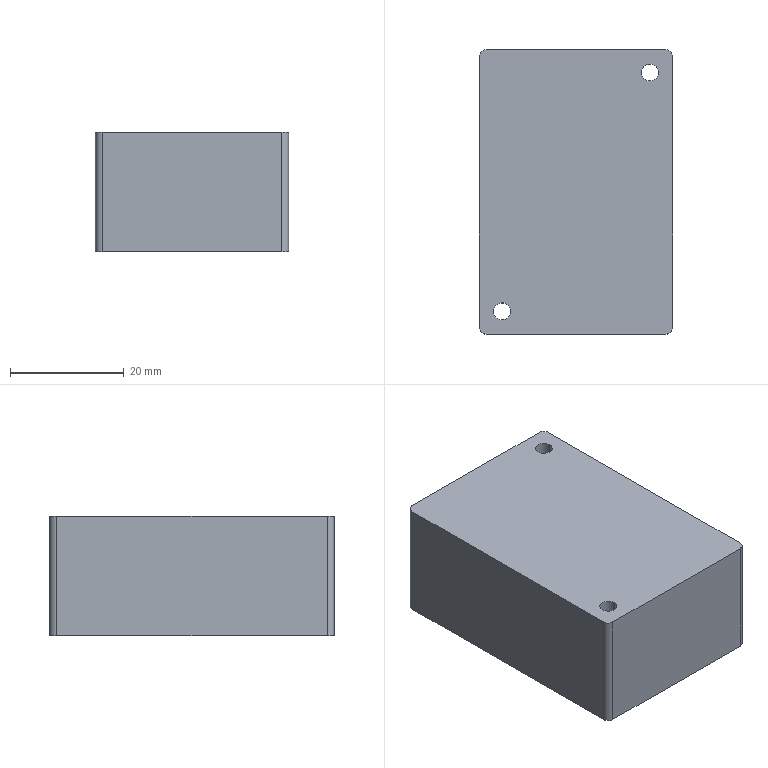Part | STEP file | 4V430C_15_Valve_Cover | 1 solid | 14 faces | box 34 x 50 x 21 mm | volume 35377 mm3 | cylinder 8 | plane 6 | commonest cylinder face diameters 2.4 x4 3 x4
STEP:
#1=CARTESIAN_POINT('',(0.,0.,0.));
#2=DIRECTION('',(0.,0.,1.));
#3=DIRECTION('',(1.,0.,0.));
#4=AXIS2_PLACEMENT_3D('',#1,#2,#3);
#5=CARTESIAN_POINT('',(-11.5,-21.,-21.));
#6=VERTEX_POINT('',#5);
#7=CARTESIAN_POINT('',(-11.5,-21.,0.));
#8=VERTEX_POINT('',#7);
#9=CARTESIAN_POINT('',(-11.5,-21.,-21.));
#10=DIRECTION('',(0.,0.,1.));
#11=VECTOR('',#10,1.);
#12=LINE('',#9,#11);
#13=CARTESIAN_POINT('',(-13.,-21.,-21.));
#14=DIRECTION('',(0.,0.,1.));
#15=DIRECTION('',(1.,0.,0.));
#16=AXIS2_PLACEMENT_3D('',#13,#14,#15);
#17=CYLINDRICAL_SURFACE('',#16,1.5);
#18=CARTESIAN_POINT('',(6.283,0.));
#19=DIRECTION('',(0.,1.));
#20=VECTOR('',#19,1.);
#21=LINE('',#18,#20);
#22=(GEOMETRIC_REPRESENTATION_CONTEXT(2)PARAMETRIC_REPRESENTATION_CONTEXT()REPRESENTATION_CONTEXT('',''));
#23=DEFINITIONAL_REPRESENTATION('',(#21),#22);
#24=PCURVE('',#17,#23);
#25=CARTESIAN_POINT('',(-13.,-21.,-21.));
#26=DIRECTION('',(0.,0.,1.));
#27=DIRECTION('',(1.,0.,0.));
#28=AXIS2_PLACEMENT_3D('',#25,#26,#27);
#29=CYLINDRICAL_SURFACE('',#28,1.5);
#30=CARTESIAN_POINT('',(0.,0.));
#31=DIRECTION('',(0.,1.));
#32=VECTOR('',#31,1.);
#33=LINE('',#30,#32);
#34=(GEOMETRIC_REPRESENTATION_CONTEXT(2)PARAMETRIC_REPRESENTATION_CONTEXT()REPRESENTATION_CONTEXT('',''));
#35=DEFINITIONAL_REPRESENTATION('',(#33),#34);
#36=PCURVE('',#29,#35);
#37=SURFACE_CURVE('',#12,(#24,#36),.PCURVE_S1.);
#38=EDGE_CURVE('',#6,#8,#37,.T.);
#39=ORIENTED_EDGE('',*,*,#38,.T.);
#40=CARTESIAN_POINT('',(-14.5,-21.,0.));
#41=VERTEX_POINT('',#40);
#42=CARTESIAN_POINT('',(-13.,-21.,0.));
#43=DIRECTION('',(0.,0.,1.));
#44=DIRECTION('',(1.,0.,0.));
#45=AXIS2_PLACEMENT_3D('',#42,#43,#44);
#46=CIRCLE('',#45,1.5);
#47=CARTESIAN_POINT('',(0.,21.));
#48=DIRECTION('',(1.,0.));
#49=VECTOR('',#48,1.);
#50=LINE('',#47,#49);
#51=(GEOMETRIC_REPRESENTATION_CONTEXT(2)PARAMETRIC_REPRESENTATION_CONTEXT()REPRESENTATION_CONTEXT('',''));
#52=DEFINITIONAL_REPRESENTATION('',(#50),#51);
#53=PCURVE('',#17,#52);
#54=CARTESIAN_POINT('',(-15.8,-23.8,0.));
#55=DIRECTION('',(0.,0.,1.));
#56=DIRECTION('',(1.,0.,0.));
#57=AXIS2_PLACEMENT_3D('',#54,#55,#56);
#58=PLANE('',#57);
#59=CARTESIAN_POINT('',(2.8,2.8));
#60=DIRECTION('',(1.,0.));
#61=AXIS2_PLACEMENT_2D('',#59,#60);
#62=CIRCLE('',#61,1.5);
#63=(GEOMETRIC_REPRESENTATION_CONTEXT(2)PARAMETRIC_REPRESENTATION_CONTEXT()REPRESENTATION_CONTEXT('',''));
#64=DEFINITIONAL_REPRESENTATION('',(#62),#63);
#65=PCURVE('',#58,#64);
#66=SURFACE_CURVE('',#46,(#53,#65),.PCURVE_S1.);
#67=EDGE_CURVE('',#41,#8,#66,.T.);
#68=ORIENTED_EDGE('',*,*,#67,.F.);
#69=CARTESIAN_POINT('',(-14.5,-21.,-21.));
#70=VERTEX_POINT('',#69);
#71=CARTESIAN_POINT('',(-14.5,-21.,-21.));
#72=DIRECTION('',(0.,0.,1.));
#73=VECTOR('',#72,1.);
#74=LINE('',#71,#73);
#75=CARTESIAN_POINT('',(3.142,0.));
#76=DIRECTION('',(0.,1.));
#77=VECTOR('',#76,1.);
#78=LINE('',#75,#77);
#79=(GEOMETRIC_REPRESENTATION_CONTEXT(2)PARAMETRIC_REPRESENTATION_CONTEXT()REPRESENTATION_CONTEXT('',''));
#80=DEFINITIONAL_REPRESENTATION('',(#78),#79);
#81=PCURVE('',#17,#80);
#82=CARTESIAN_POINT('',(3.142,0.));
#83=DIRECTION('',(0.,1.));
#84=VECTOR('',#83,1.);
#85=LINE('',#82,#84);
#86=(GEOMETRIC_REPRESENTATION_CONTEXT(2)PARAMETRIC_REPRESENTATION_CONTEXT()REPRESENTATION_CONTEXT('',''));
#87=DEFINITIONAL_REPRESENTATION('',(#85),#86);
#88=PCURVE('',#29,#87);
#89=SURFACE_CURVE('',#74,(#81,#88),.PCURVE_S1.);
#90=EDGE_CURVE('',#70,#41,#89,.T.);
#91=ORIENTED_EDGE('',*,*,#90,.F.);
#92=CARTESIAN_POINT('',(-13.,-21.,-21.));
#93=DIRECTION('',(0.,0.,1.));
#94=DIRECTION('',(1.,0.,0.));
#95=AXIS2_PLACEMENT_3D('',#92,#93,#94);
#96=CIRCLE('',#95,1.5);
#97=CARTESIAN_POINT('',(0.,0.));
#98=DIRECTION('',(1.,0.));
#99=VECTOR('',#98,1.);
#100=LINE('',#97,#99);
#101=(GEOMETRIC_REPRESENTATION_CONTEXT(2)PARAMETRIC_REPRESENTATION_CONTEXT()REPRESENTATION_CONTEXT('',''));
#102=DEFINITIONAL_REPRESENTATION('',(#100),#101);
#103=PCURVE('',#17,#102);
#104=CARTESIAN_POINT('',(-15.8,-23.8,-21.));
#105=DIRECTION('',(0.,0.,1.));
#106=DIRECTION('',(1.,0.,0.));
#107=AXIS2_PLACEMENT_3D('',#104,#105,#106);
#108=PLANE('',#107);
#109=CARTESIAN_POINT('',(2.8,2.8));
#110=DIRECTION('',(1.,0.));
#111=AXIS2_PLACEMENT_2D('',#109,#110);
#112=CIRCLE('',#111,1.5);
#113=(GEOMETRIC_REPRESENTATION_CONTEXT(2)PARAMETRIC_REPRESENTATION_CONTEXT()REPRESENTATION_CONTEXT('',''));
#114=DEFINITIONAL_REPRESENTATION('',(#112),#113);
#115=PCURVE('',#108,#114);
#116=SURFACE_CURVE('',#96,(#103,#115),.PCURVE_S1.);
#117=EDGE_CURVE('',#70,#6,#116,.T.);
#118=ORIENTED_EDGE('',*,*,#117,.T.);
#119=EDGE_LOOP('',(#39,#68,#91,#118));
#120=FACE_BOUND('',#119,.F.);
#121=ADVANCED_FACE('',(#120),#17,.F.);
#122=CARTESIAN_POINT('',(14.5,21.,-21.));
#123=VERTEX_POINT('',#122);
#124=CARTESIAN_POINT('',(14.5,21.,0.));
#125=VERTEX_POINT('',#124);
#126=CARTESIAN_POINT('',(14.5,21.,-21.));
#127=DIRECTION('',(0.,0.,1.));
#128=VECTOR('',#127,1.);
#129=LINE('',#126,#128);
#130=CARTESIAN_POINT('',(13.,21.,-21.));
#131=DIRECTION('',(0.,0.,1.));
#132=DIRECTION('',(1.,0.,0.));
#133=AXIS2_PLACEMENT_3D('',#130,#131,#132);
#134=CYLINDRICAL_SURFACE('',#133,1.5);
#135=CARTESIAN_POINT('',(6.283,0.));
#136=DIRECTION('',(0.,1.));
#137=VECTOR('',#136,1.);
#138=LINE('',#135,#137);
#139=(GEOMETRIC_REPRESENTATION_CONTEXT(2)PARAMETRIC_REPRESENTATION_CONTEXT()REPRESENTATION_CONTEXT('',''));
#140=DEFINITIONAL_REPRESENTATION('',(#138),#139);
#141=PCURVE('',#134,#140);
#142=CARTESIAN_POINT('',(13.,21.,-21.));
#143=DIRECTION('',(0.,0.,1.));
#144=DIRECTION('',(1.,0.,0.));
#145=AXIS2_PLACEMENT_3D('',#142,#143,#144);
#146=CYLINDRICAL_SURFACE('',#145,1.5);
#147=CARTESIAN_POINT('',(0.,0.));
#148=DIRECTION('',(0.,1.));
#149=VECTOR('',#148,1.);
#150=LINE('',#147,#149);
#151=(GEOMETRIC_REPRESENTATION_CONTEXT(2)PARAMETRIC_REPRESENTATION_CONTEXT()REPRESENTATION_CONTEXT('',''));
#152=DEFINITIONAL_REPRESENTATION('',(#150),#151);
#153=PCURVE('',#146,#152);
#154=SURFACE_CURVE('',#129,(#141,#153),.PCURVE_S1.);
#155=EDGE_CURVE('',#123,#125,#154,.T.);
#156=ORIENTED_EDGE('',*,*,#155,.T.);
#157=CARTESIAN_POINT('',(11.5,21.,0.));
#158=VERTEX_POINT('',#157);
#159=CARTESIAN_POINT('',(13.,21.,0.));
#160=DIRECTION('',(0.,0.,1.));
#161=DIRECTION('',(1.,0.,0.));
#162=AXIS2_PLACEMENT_3D('',#159,#160,#161);
#163=CIRCLE('',#162,1.5);
#164=CARTESIAN_POINT('',(0.,21.));
#165=DIRECTION('',(1.,0.));
#166=VECTOR('',#165,1.);
#167=LINE('',#164,#166);
#168=(GEOMETRIC_REPRESENTATION_CONTEXT(2)PARAMETRIC_REPRESENTATION_CONTEXT()REPRESENTATION_CONTEXT('',''));
#169=DEFINITIONAL_REPRESENTATION('',(#167),#168);
#170=PCURVE('',#134,#169);
#171=CARTESIAN_POINT('',(28.8,44.8));
#172=DIRECTION('',(1.,0.));
#173=AXIS2_PLACEMENT_2D('',#171,#172);
#174=CIRCLE('',#173,1.5);
#175=(GEOMETRIC_REPRESENTATION_CONTEXT(2)PARAMETRIC_REPRESENTATION_CONTEXT()REPRESENTATION_CONTEXT('',''));
#176=DEFINITIONAL_REPRESENTATION('',(#174),#175);
#177=PCURVE('',#58,#176);
#178=SURFACE_CURVE('',#163,(#170,#177),.PCURVE_S1.);
#179=EDGE_CURVE('',#158,#125,#178,.T.);
#180=ORIENTED_EDGE('',*,*,#179,.F.);
#181=CARTESIAN_POINT('',(11.5,21.,-21.));
#182=VERTEX_POINT('',#181);
#183=CARTESIAN_POINT('',(11.5,21.,-21.));
#184=DIRECTION('',(0.,0.,1.));
#185=VECTOR('',#184,1.);
#186=LINE('',#183,#185);
#187=CARTESIAN_POINT('',(3.142,0.));
#188=DIRECTION('',(0.,1.));
#189=VECTOR('',#188,1.);
#190=LINE('',#187,#189);
#191=(GEOMETRIC_REPRESENTATION_CONTEXT(2)PARAMETRIC_REPRESENTATION_CONTEXT()REPRESENTATION_CONTEXT('',''));
#192=DEFINITIONAL_REPRESENTATION('',(#190),#191);
#193=PCURVE('',#134,#192);
#194=CARTESIAN_POINT('',(3.142,0.));
#195=DIRECTION('',(0.,1.));
#196=VECTOR('',#195,1.);
#197=LINE('',#194,#196);
#198=(GEOMETRIC_REPRESENTATION_CONTEXT(2)PARAMETRIC_REPRESENTATION_CONTEXT()REPRESENTATION_CONTEXT('',''));
#199=DEFINITIONAL_REPRESENTATION('',(#197),#198);
#200=PCURVE('',#146,#199);
#201=SURFACE_CURVE('',#186,(#193,#200),.PCURVE_S1.);
#202=EDGE_CURVE('',#182,#158,#201,.T.);
#203=ORIENTED_EDGE('',*,*,#202,.F.);
#204=CARTESIAN_POINT('',(13.,21.,-21.));
#205=DIRECTION('',(0.,0.,1.));
#206=DIRECTION('',(1.,0.,0.));
#207=AXIS2_PLACEMENT_3D('',#204,#205,#206);
#208=CIRCLE('',#207,1.5);
#209=CARTESIAN_POINT('',(0.,0.));
#210=DIRECTION('',(1.,0.));
#211=VECTOR('',#210,1.);
#212=LINE('',#209,#211);
#213=(GEOMETRIC_REPRESENTATION_CONTEXT(2)PARAMETRIC_REPRESENTATION_CONTEXT()REPRESENTATION_CONTEXT('',''));
#214=DEFINITIONAL_REPRESENTATION('',(#212),#213);
#215=PCURVE('',#134,#214);
#216=CARTESIAN_POINT('',(28.8,44.8));
#217=DIRECTION('',(1.,0.));
#218=AXIS2_PLACEMENT_2D('',#216,#217);
#219=CIRCLE('',#218,1.5);
#220=(GEOMETRIC_REPRESENTATION_CONTEXT(2)PARAMETRIC_REPRESENTATION_CONTEXT()REPRESENTATION_CONTEXT('',''));
#221=DEFINITIONAL_REPRESENTATION('',(#219),#220);
#222=PCURVE('',#108,#221);
#223=SURFACE_CURVE('',#208,(#215,#222),.PCURVE_S1.);
#224=EDGE_CURVE('',#182,#123,#223,.T.);
#225=ORIENTED_EDGE('',*,*,#224,.T.);
#226=EDGE_LOOP('',(#156,#180,#203,#225));
#227=FACE_BOUND('',#226,.F.);
#228=ADVANCED_FACE('',(#227),#134,.F.);
#229=CARTESIAN_POINT('',(-17.,-23.8,0.));
#230=VERTEX_POINT('',#229);
#231=CARTESIAN_POINT('',(-15.8,-25.,0.));
#232=VERTEX_POINT('',#231);
#233=CARTESIAN_POINT('',(-15.8,-23.8,0.));
#234=DIRECTION('',(0.,0.,1.));
#235=DIRECTION('',(1.,0.,0.));
#236=AXIS2_PLACEMENT_3D('',#233,#234,#235);
#237=CIRCLE('',#236,1.2);
#238=CARTESIAN_POINT('',(-15.8,-23.8,-21.));
#239=DIRECTION('',(0.,0.,1.));
#240=DIRECTION('',(1.,0.,0.));
#241=AXIS2_PLACEMENT_3D('',#238,#239,#240);
#242=CYLINDRICAL_SURFACE('',#241,1.2);
#243=CARTESIAN_POINT('',(0.,21.));
#244=DIRECTION('',(1.,0.));
#245=VECTOR('',#244,1.);
#246=LINE('',#243,#245);
#247=(GEOMETRIC_REPRESENTATION_CONTEXT(2)PARAMETRIC_REPRESENTATION_CONTEXT()REPRESENTATION_CONTEXT('',''));
#248=DEFINITIONAL_REPRESENTATION('',(#246),#247);
#249=PCURVE('',#242,#248);
#250=CARTESIAN_POINT('',(0.,0.));
#251=DIRECTION('',(1.,0.));
#252=AXIS2_PLACEMENT_2D('',#250,#251);
#253=CIRCLE('',#252,1.2);
#254=(GEOMETRIC_REPRESENTATION_CONTEXT(2)PARAMETRIC_REPRESENTATION_CONTEXT()REPRESENTATION_CONTEXT('',''));
#255=DEFINITIONAL_REPRESENTATION('',(#253),#254);
#256=PCURVE('',#58,#255);
#257=SURFACE_CURVE('',#237,(#249,#256),.PCURVE_S1.);
#258=EDGE_CURVE('',#230,#232,#257,.T.);
#259=ORIENTED_EDGE('',*,*,#258,.F.);
#260=CARTESIAN_POINT('',(-17.,-23.8,-21.));
#261=VERTEX_POINT('',#260);
#262=CARTESIAN_POINT('',(-17.,-23.8,-21.));
#263=DIRECTION('',(0.,0.,1.));
#264=VECTOR('',#263,1.);
#265=LINE('',#262,#264);
#266=CARTESIAN_POINT('',(3.142,0.));
#267=DIRECTION('',(0.,1.));
#268=VECTOR('',#267,1.);
#269=LINE('',#266,#268);
#270=(GEOMETRIC_REPRESENTATION_CONTEXT(2)PARAMETRIC_REPRESENTATION_CONTEXT()REPRESENTATION_CONTEXT('',''));
#271=DEFINITIONAL_REPRESENTATION('',(#269),#270);
#272=PCURVE('',#242,#271);
#273=CARTESIAN_POINT('',(-17.,23.8,-21.));
#274=DIRECTION('',(-1.,0.,0.));
#275=DIRECTION('',(0.,0.,1.));
#276=AXIS2_PLACEMENT_3D('',#273,#274,#275);
#277=PLANE('',#276);
#278=CARTESIAN_POINT('',(0.,-47.6));
#279=DIRECTION('',(1.,0.));
#280=VECTOR('',#279,1.);
#281=LINE('',#278,#280);
#282=(GEOMETRIC_REPRESENTATION_CONTEXT(2)PARAMETRIC_REPRESENTATION_CONTEXT()REPRESENTATION_CONTEXT('',''));
#283=DEFINITIONAL_REPRESENTATION('',(#281),#282);
#284=PCURVE('',#277,#283);
#285=SURFACE_CURVE('',#265,(#272,#284),.PCURVE_S1.);
#286=EDGE_CURVE('',#261,#230,#285,.T.);
#287=ORIENTED_EDGE('',*,*,#286,.F.);
#288=CARTESIAN_POINT('',(-15.8,-25.,-21.));
#289=VERTEX_POINT('',#288);
#290=CARTESIAN_POINT('',(-15.8,-23.8,-21.));
#291=DIRECTION('',(0.,0.,1.));
#292=DIRECTION('',(1.,0.,0.));
#293=AXIS2_PLACEMENT_3D('',#290,#291,#292);
#294=CIRCLE('',#293,1.2);
#295=CARTESIAN_POINT('',(0.,0.));
#296=DIRECTION('',(1.,0.));
#297=VECTOR('',#296,1.);
#298=LINE('',#295,#297);
#299=(GEOMETRIC_REPRESENTATION_CONTEXT(2)PARAMETRIC_REPRESENTATION_CONTEXT()REPRESENTATION_CONTEXT('',''));
#300=DEFINITIONAL_REPRESENTATION('',(#298),#299);
#301=PCURVE('',#242,#300);
#302=CARTESIAN_POINT('',(0.,0.));
#303=DIRECTION('',(1.,0.));
#304=AXIS2_PLACEMENT_2D('',#302,#303);
#305=CIRCLE('',#304,1.2);
#306=(GEOMETRIC_REPRESENTATION_CONTEXT(2)PARAMETRIC_REPRESENTATION_CONTEXT()REPRESENTATION_CONTEXT('',''));
#307=DEFINITIONAL_REPRESENTATION('',(#305),#306);
#308=PCURVE('',#108,#307);
#309=SURFACE_CURVE('',#294,(#301,#308),.PCURVE_S1.);
#310=EDGE_CURVE('',#261,#289,#309,.T.);
#311=ORIENTED_EDGE('',*,*,#310,.T.);
#312=CARTESIAN_POINT('',(-15.8,-25.,-21.));
#313=DIRECTION('',(0.,0.,1.));
#314=VECTOR('',#313,1.);
#315=LINE('',#312,#314);
#316=CARTESIAN_POINT('',(4.712,0.));
#317=DIRECTION('',(0.,1.));
#318=VECTOR('',#317,1.);
#319=LINE('',#316,#318);
#320=(GEOMETRIC_REPRESENTATION_CONTEXT(2)PARAMETRIC_REPRESENTATION_CONTEXT()REPRESENTATION_CONTEXT('',''));
#321=DEFINITIONAL_REPRESENTATION('',(#319),#320);
#322=PCURVE('',#242,#321);
#323=CARTESIAN_POINT('',(-15.8,-25.,-21.));
#324=DIRECTION('',(0.,-1.,0.));
#325=DIRECTION('',(0.,0.,-1.));
#326=AXIS2_PLACEMENT_3D('',#323,#324,#325);
#327=PLANE('',#326);
#328=CARTESIAN_POINT('',(0.,0.));
#329=DIRECTION('',(-1.,0.));
#330=VECTOR('',#329,1.);
#331=LINE('',#328,#330);
#332=(GEOMETRIC_REPRESENTATION_CONTEXT(2)PARAMETRIC_REPRESENTATION_CONTEXT()REPRESENTATION_CONTEXT('',''));
#333=DEFINITIONAL_REPRESENTATION('',(#331),#332);
#334=PCURVE('',#327,#333);
#335=SURFACE_CURVE('',#315,(#322,#334),.PCURVE_S1.);
#336=EDGE_CURVE('',#289,#232,#335,.T.);
#337=ORIENTED_EDGE('',*,*,#336,.T.);
#338=EDGE_LOOP('',(#259,#287,#311,#337));
#339=FACE_BOUND('',#338,.T.);
#340=ADVANCED_FACE('',(#339),#242,.T.);
#341=CARTESIAN_POINT('',(-17.,23.8,0.));
#342=VERTEX_POINT('',#341);
#343=CARTESIAN_POINT('',(-17.,23.8,0.));
#344=DIRECTION('',(0.,-1.,0.));
#345=VECTOR('',#344,1.);
#346=LINE('',#343,#345);
#347=CARTESIAN_POINT('',(21.,0.));
#348=DIRECTION('',(0.,-1.));
#349=VECTOR('',#348,1.);
#350=LINE('',#347,#349);
#351=(GEOMETRIC_REPRESENTATION_CONTEXT(2)PARAMETRIC_REPRESENTATION_CONTEXT()REPRESENTATION_CONTEXT('',''));
#352=DEFINITIONAL_REPRESENTATION('',(#350),#351);
#353=PCURVE('',#277,#352);
#354=CARTESIAN_POINT('',(-1.2,47.6));
#355=DIRECTION('',(0.,-1.));
#356=VECTOR('',#355,1.);
#357=LINE('',#354,#356);
#358=(GEOMETRIC_REPRESENTATION_CONTEXT(2)PARAMETRIC_REPRESENTATION_CONTEXT()REPRESENTATION_CONTEXT('',''));
#359=DEFINITIONAL_REPRESENTATION('',(#357),#358);
#360=PCURVE('',#58,#359);
#361=SURFACE_CURVE('',#346,(#353,#360),.PCURVE_S1.);
#362=EDGE_CURVE('',#342,#230,#361,.T.);
#363=ORIENTED_EDGE('',*,*,#362,.F.);
#364=CARTESIAN_POINT('',(-17.,23.8,-21.));
#365=VERTEX_POINT('',#364);
#366=CARTESIAN_POINT('',(-17.,23.8,-21.));
#367=DIRECTION('',(0.,0.,1.));
#368=VECTOR('',#367,1.);
#369=LINE('',#366,#368);
#370=CARTESIAN_POINT('',(0.,0.));
#371=DIRECTION('',(1.,0.));
#372=VECTOR('',#371,1.);
#373=LINE('',#370,#372);
#374=(GEOMETRIC_REPRESENTATION_CONTEXT(2)PARAMETRIC_REPRESENTATION_CONTEXT()REPRESENTATION_CONTEXT('',''));
#375=DEFINITIONAL_REPRESENTATION('',(#373),#374);
#376=PCURVE('',#277,#375);
#377=CARTESIAN_POINT('',(-15.8,23.8,-21.));
#378=DIRECTION('',(0.,0.,1.));
#379=DIRECTION('',(1.,0.,0.));
#380=AXIS2_PLACEMENT_3D('',#377,#378,#379);
#381=CYLINDRICAL_SURFACE('',#380,1.2);
#382=CARTESIAN_POINT('',(3.142,0.));
#383=DIRECTION('',(0.,1.));
#384=VECTOR('',#383,1.);
#385=LINE('',#382,#384);
#386=(GEOMETRIC_REPRESENTATION_CONTEXT(2)PARAMETRIC_REPRESENTATION_CONTEXT()REPRESENTATION_CONTEXT('',''));
#387=DEFINITIONAL_REPRESENTATION('',(#385),#386);
#388=PCURVE('',#381,#387);
#389=SURFACE_CURVE('',#369,(#376,#388),.PCURVE_S1.);
#390=EDGE_CURVE('',#365,#342,#389,.T.);
#391=ORIENTED_EDGE('',*,*,#390,.F.);
#392=CARTESIAN_POINT('',(-17.,23.8,-21.));
#393=DIRECTION('',(0.,-1.,0.));
#394=VECTOR('',#393,1.);
#395=LINE('',#392,#394);
#396=CARTESIAN_POINT('',(0.,0.));
#397=DIRECTION('',(0.,-1.));
#398=VECTOR('',#397,1.);
#399=LINE('',#396,#398);
#400=(GEOMETRIC_REPRESENTATION_CONTEXT(2)PARAMETRIC_REPRESENTATION_CONTEXT()REPRESENTATION_CONTEXT('',''));
#401=DEFINITIONAL_REPRESENTATION('',(#399),#400);
#402=PCURVE('',#277,#401);
#403=CARTESIAN_POINT('',(-1.2,47.6));
#404=DIRECTION('',(0.,-1.));
#405=VECTOR('',#404,1.);
#406=LINE('',#403,#405);
#407=(GEOMETRIC_REPRESENTATION_CONTEXT(2)PARAMETRIC_REPRESENTATION_CONTEXT()REPRESENTATION_CONTEXT('',''));
#408=DEFINITIONAL_REPRESENTATION('',(#406),#407);
#409=PCURVE('',#108,#408);
#410=SURFACE_CURVE('',#395,(#402,#409),.PCURVE_S1.);
#411=EDGE_CURVE('',#365,#261,#410,.T.);
#412=ORIENTED_EDGE('',*,*,#411,.T.);
#413=ORIENTED_EDGE('',*,*,#286,.T.);
#414=EDGE_LOOP('',(#363,#391,#412,#413));
#415=FACE_BOUND('',#414,.T.);
#416=ADVANCED_FACE('',(#415),#277,.T.);
#417=CARTESIAN_POINT('',(-15.8,25.,0.));
#418=VERTEX_POINT('',#417);
#419=CARTESIAN_POINT('',(-15.8,23.8,0.));
#420=DIRECTION('',(0.,0.,1.));
#421=DIRECTION('',(1.,0.,0.));
#422=AXIS2_PLACEMENT_3D('',#419,#420,#421);
#423=CIRCLE('',#422,1.2);
#424=CARTESIAN_POINT('',(0.,21.));
#425=DIRECTION('',(1.,0.));
#426=VECTOR('',#425,1.);
#427=LINE('',#424,#426);
#428=(GEOMETRIC_REPRESENTATION_CONTEXT(2)PARAMETRIC_REPRESENTATION_CONTEXT()REPRESENTATION_CONTEXT('',''));
#429=DEFINITIONAL_REPRESENTATION('',(#427),#428);
#430=PCURVE('',#381,#429);
#431=CARTESIAN_POINT('',(0.,47.6));
#432=DIRECTION('',(1.,0.));
#433=AXIS2_PLACEMENT_2D('',#431,#432);
#434=CIRCLE('',#433,1.2);
#435=(GEOMETRIC_REPRESENTATION_CONTEXT(2)PARAMETRIC_REPRESENTATION_CONTEXT()REPRESENTATION_CONTEXT('',''));
#436=DEFINITIONAL_REPRESENTATION('',(#434),#435);
#437=PCURVE('',#58,#436);
#438=SURFACE_CURVE('',#423,(#430,#437),.PCURVE_S1.);
#439=EDGE_CURVE('',#418,#342,#438,.T.);
#440=ORIENTED_EDGE('',*,*,#439,.F.);
#441=CARTESIAN_POINT('',(-15.8,25.,-21.));
#442=VERTEX_POINT('',#441);
#443=CARTESIAN_POINT('',(-15.8,25.,-21.));
#444=DIRECTION('',(0.,0.,1.));
#445=VECTOR('',#444,1.);
#446=LINE('',#443,#445);
#447=CARTESIAN_POINT('',(1.571,0.));
#448=DIRECTION('',(0.,1.));
#449=VECTOR('',#448,1.);
#450=LINE('',#447,#449);
#451=(GEOMETRIC_REPRESENTATION_CONTEXT(2)PARAMETRIC_REPRESENTATION_CONTEXT()REPRESENTATION_CONTEXT('',''));
#452=DEFINITIONAL_REPRESENTATION('',(#450),#451);
#453=PCURVE('',#381,#452);
#454=CARTESIAN_POINT('',(15.8,25.,-21.));
#455=DIRECTION('',(0.,1.,0.));
#456=DIRECTION('',(0.,0.,1.));
#457=AXIS2_PLACEMENT_3D('',#454,#455,#456);
#458=PLANE('',#457);
#459=CARTESIAN_POINT('',(0.,-31.6));
#460=DIRECTION('',(1.,0.));
#461=VECTOR('',#460,1.);
#462=LINE('',#459,#461);
#463=(GEOMETRIC_REPRESENTATION_CONTEXT(2)PARAMETRIC_REPRESENTATION_CONTEXT()REPRESENTATION_CONTEXT('',''));
#464=DEFINITIONAL_REPRESENTATION('',(#462),#463);
#465=PCURVE('',#458,#464);
#466=SURFACE_CURVE('',#446,(#453,#465),.PCURVE_S1.);
#467=EDGE_CURVE('',#442,#418,#466,.T.);
#468=ORIENTED_EDGE('',*,*,#467,.F.);
#469=CARTESIAN_POINT('',(-15.8,23.8,-21.));
#470=DIRECTION('',(0.,0.,1.));
#471=DIRECTION('',(1.,0.,0.));
#472=AXIS2_PLACEMENT_3D('',#469,#470,#471);
#473=CIRCLE('',#472,1.2);
#474=CARTESIAN_POINT('',(0.,0.));
#475=DIRECTION('',(1.,0.));
#476=VECTOR('',#475,1.);
#477=LINE('',#474,#476);
#478=(GEOMETRIC_REPRESENTATION_CONTEXT(2)PARAMETRIC_REPRESENTATION_CONTEXT()REPRESENTATION_CONTEXT('',''));
#479=DEFINITIONAL_REPRESENTATION('',(#477),#478);
#480=PCURVE('',#381,#479);
#481=CARTESIAN_POINT('',(0.,47.6));
#482=DIRECTION('',(1.,0.));
#483=AXIS2_PLACEMENT_2D('',#481,#482);
#484=CIRCLE('',#483,1.2);
#485=(GEOMETRIC_REPRESENTATION_CONTEXT(2)PARAMETRIC_REPRESENTATION_CONTEXT()REPRESENTATION_CONTEXT('',''));
#486=DEFINITIONAL_REPRESENTATION('',(#484),#485);
#487=PCURVE('',#108,#486);
#488=SURFACE_CURVE('',#473,(#480,#487),.PCURVE_S1.);
#489=EDGE_CURVE('',#442,#365,#488,.T.);
#490=ORIENTED_EDGE('',*,*,#489,.T.);
#491=ORIENTED_EDGE('',*,*,#390,.T.);
#492=EDGE_LOOP('',(#440,#468,#490,#491));
#493=FACE_BOUND('',#492,.T.);
#494=ADVANCED_FACE('',(#493),#381,.T.);
#495=CARTESIAN_POINT('',(15.8,25.,0.));
#496=VERTEX_POINT('',#495);
#497=CARTESIAN_POINT('',(15.8,25.,0.));
#498=DIRECTION('',(-1.,0.,0.));
#499=VECTOR('',#498,1.);
#500=LINE('',#497,#499);
#501=CARTESIAN_POINT('',(21.,0.));
#502=DIRECTION('',(0.,-1.));
#503=VECTOR('',#502,1.);
#504=LINE('',#501,#503);
#505=(GEOMETRIC_REPRESENTATION_CONTEXT(2)PARAMETRIC_REPRESENTATION_CONTEXT()REPRESENTATION_CONTEXT('',''));
#506=DEFINITIONAL_REPRESENTATION('',(#504),#505);
#507=PCURVE('',#458,#506);
#508=CARTESIAN_POINT('',(31.6,48.8));
#509=DIRECTION('',(-1.,0.));
#510=VECTOR('',#509,1.);
#511=LINE('',#508,#510);
#512=(GEOMETRIC_REPRESENTATION_CONTEXT(2)PARAMETRIC_REPRESENTATION_CONTEXT()REPRESENTATION_CONTEXT('',''));
#513=DEFINITIONAL_REPRESENTATION('',(#511),#512);
#514=PCURVE('',#58,#513);
#515=SURFACE_CURVE('',#500,(#507,#514),.PCURVE_S1.);
#516=EDGE_CURVE('',#496,#418,#515,.T.);
#517=ORIENTED_EDGE('',*,*,#516,.F.);
#518=CARTESIAN_POINT('',(15.8,25.,-21.));
#519=VERTEX_POINT('',#518);
#520=CARTESIAN_POINT('',(15.8,25.,-21.));
#521=DIRECTION('',(0.,0.,1.));
#522=VECTOR('',#521,1.);
#523=LINE('',#520,#522);
#524=CARTESIAN_POINT('',(0.,0.));
#525=DIRECTION('',(1.,0.));
#526=VECTOR('',#525,1.);
#527=LINE('',#524,#526);
#528=(GEOMETRIC_REPRESENTATION_CONTEXT(2)PARAMETRIC_REPRESENTATION_CONTEXT()REPRESENTATION_CONTEXT('',''));
#529=DEFINITIONAL_REPRESENTATION('',(#527),#528);
#530=PCURVE('',#458,#529);
#531=CARTESIAN_POINT('',(15.8,23.8,-21.));
#532=DIRECTION('',(0.,0.,1.));
#533=DIRECTION('',(1.,0.,0.));
#534=AXIS2_PLACEMENT_3D('',#531,#532,#533);
#535=CYLINDRICAL_SURFACE('',#534,1.2);
#536=CARTESIAN_POINT('',(1.571,0.));
#537=DIRECTION('',(0.,1.));
#538=VECTOR('',#537,1.);
#539=LINE('',#536,#538);
#540=(GEOMETRIC_REPRESENTATION_CONTEXT(2)PARAMETRIC_REPRESENTATION_CONTEXT()REPRESENTATION_CONTEXT('',''));
#541=DEFINITIONAL_REPRESENTATION('',(#539),#540);
#542=PCURVE('',#535,#541);
#543=SURFACE_CURVE('',#523,(#530,#542),.PCURVE_S1.);
#544=EDGE_CURVE('',#519,#496,#543,.T.);
#545=ORIENTED_EDGE('',*,*,#544,.F.);
#546=CARTESIAN_POINT('',(15.8,25.,-21.));
#547=DIRECTION('',(-1.,0.,0.));
#548=VECTOR('',#547,1.);
#549=LINE('',#546,#548);
#550=CARTESIAN_POINT('',(0.,0.));
#551=DIRECTION('',(0.,-1.));
#552=VECTOR('',#551,1.);
#553=LINE('',#550,#552);
#554=(GEOMETRIC_REPRESENTATION_CONTEXT(2)PARAMETRIC_REPRESENTATION_CONTEXT()REPRESENTATION_CONTEXT('',''));
#555=DEFINITIONAL_REPRESENTATION('',(#553),#554);
#556=PCURVE('',#458,#555);
#557=CARTESIAN_POINT('',(31.6,48.8));
#558=DIRECTION('',(-1.,0.));
#559=VECTOR('',#558,1.);
#560=LINE('',#557,#559);
#561=(GEOMETRIC_REPRESENTATION_CONTEXT(2)PARAMETRIC_REPRESENTATION_CONTEXT()REPRESENTATION_CONTEXT('',''));
#562=DEFINITIONAL_REPRESENTATION('',(#560),#561);
#563=PCURVE('',#108,#562);
#564=SURFACE_CURVE('',#549,(#556,#563),.PCURVE_S1.);
#565=EDGE_CURVE('',#519,#442,#564,.T.);
#566=ORIENTED_EDGE('',*,*,#565,.T.);
#567=ORIENTED_EDGE('',*,*,#467,.T.);
#568=EDGE_LOOP('',(#517,#545,#566,#567));
#569=FACE_BOUND('',#568,.T.);
#570=ADVANCED_FACE('',(#569),#458,.T.);
#571=CARTESIAN_POINT('',(17.,23.8,0.));
#572=VERTEX_POINT('',#571);
#573=CARTESIAN_POINT('',(15.8,23.8,0.));
#574=DIRECTION('',(0.,0.,1.));
#575=DIRECTION('',(1.,0.,0.));
#576=AXIS2_PLACEMENT_3D('',#573,#574,#575);
#577=CIRCLE('',#576,1.2);
#578=CARTESIAN_POINT('',(0.,21.));
#579=DIRECTION('',(1.,0.));
#580=VECTOR('',#579,1.);
#581=LINE('',#578,#580);
#582=(GEOMETRIC_REPRESENTATION_CONTEXT(2)PARAMETRIC_REPRESENTATION_CONTEXT()REPRESENTATION_CONTEXT('',''));
#583=DEFINITIONAL_REPRESENTATION('',(#581),#582);
#584=PCURVE('',#535,#583);
#585=CARTESIAN_POINT('',(31.6,47.6));
#586=DIRECTION('',(1.,0.));
#587=AXIS2_PLACEMENT_2D('',#585,#586);
#588=CIRCLE('',#587,1.2);
#589=(GEOMETRIC_REPRESENTATION_CONTEXT(2)PARAMETRIC_REPRESENTATION_CONTEXT()REPRESENTATION_CONTEXT('',''));
#590=DEFINITIONAL_REPRESENTATION('',(#588),#589);
#591=PCURVE('',#58,#590);
#592=SURFACE_CURVE('',#577,(#584,#591),.PCURVE_S1.);
#593=EDGE_CURVE('',#572,#496,#592,.T.);
#594=ORIENTED_EDGE('',*,*,#593,.F.);
#595=CARTESIAN_POINT('',(17.,23.8,-21.));
#596=VERTEX_POINT('',#595);
#597=CARTESIAN_POINT('',(17.,23.8,-21.));
#598=DIRECTION('',(0.,0.,1.));
#599=VECTOR('',#598,1.);
#600=LINE('',#597,#599);
#601=CARTESIAN_POINT('',(0.,0.));
#602=DIRECTION('',(0.,1.));
#603=VECTOR('',#602,1.);
#604=LINE('',#601,#603);
#605=(GEOMETRIC_REPRESENTATION_CONTEXT(2)PARAMETRIC_REPRESENTATION_CONTEXT()REPRESENTATION_CONTEXT('',''));
#606=DEFINITIONAL_REPRESENTATION('',(#604),#605);
#607=PCURVE('',#535,#606);
#608=CARTESIAN_POINT('',(17.,-23.8,-21.));
#609=DIRECTION('',(1.,0.,0.));
#610=DIRECTION('',(0.,0.,-1.));
#611=AXIS2_PLACEMENT_3D('',#608,#609,#610);
#612=PLANE('',#611);
#613=CARTESIAN_POINT('',(0.,47.6));
#614=DIRECTION('',(-1.,0.));
#615=VECTOR('',#614,1.);
#616=LINE('',#613,#615);
#617=(GEOMETRIC_REPRESENTATION_CONTEXT(2)PARAMETRIC_REPRESENTATION_CONTEXT()REPRESENTATION_CONTEXT('',''));
#618=DEFINITIONAL_REPRESENTATION('',(#616),#617);
#619=PCURVE('',#612,#618);
#620=SURFACE_CURVE('',#600,(#607,#619),.PCURVE_S1.);
#621=EDGE_CURVE('',#596,#572,#620,.T.);
#622=ORIENTED_EDGE('',*,*,#621,.F.);
#623=CARTESIAN_POINT('',(15.8,23.8,-21.));
#624=DIRECTION('',(0.,0.,1.));
#625=DIRECTION('',(1.,0.,0.));
#626=AXIS2_PLACEMENT_3D('',#623,#624,#625);
#627=CIRCLE('',#626,1.2);
#628=CARTESIAN_POINT('',(0.,0.));
#629=DIRECTION('',(1.,0.));
#630=VECTOR('',#629,1.);
#631=LINE('',#628,#630);
#632=(GEOMETRIC_REPRESENTATION_CONTEXT(2)PARAMETRIC_REPRESENTATION_CONTEXT()REPRESENTATION_CONTEXT('',''));
#633=DEFINITIONAL_REPRESENTATION('',(#631),#632);
#634=PCURVE('',#535,#633);
#635=CARTESIAN_POINT('',(31.6,47.6));
#636=DIRECTION('',(1.,0.));
#637=AXIS2_PLACEMENT_2D('',#635,#636);
#638=CIRCLE('',#637,1.2);
#639=(GEOMETRIC_REPRESENTATION_CONTEXT(2)PARAMETRIC_REPRESENTATION_CONTEXT()REPRESENTATION_CONTEXT('',''));
#640=DEFINITIONAL_REPRESENTATION('',(#638),#639);
#641=PCURVE('',#108,#640);
#642=SURFACE_CURVE('',#627,(#634,#641),.PCURVE_S1.);
#643=EDGE_CURVE('',#596,#519,#642,.T.);
#644=ORIENTED_EDGE('',*,*,#643,.T.);
#645=ORIENTED_EDGE('',*,*,#544,.T.);
#646=EDGE_LOOP('',(#594,#622,#644,#645));
#647=FACE_BOUND('',#646,.T.);
#648=ADVANCED_FACE('',(#647),#535,.T.);
#649=CARTESIAN_POINT('',(17.,-23.8,0.));
#650=VERTEX_POINT('',#649);
#651=CARTESIAN_POINT('',(17.,-23.8,0.));
#652=DIRECTION('',(0.,1.,0.));
#653=VECTOR('',#652,1.);
#654=LINE('',#651,#653);
#655=CARTESIAN_POINT('',(-21.,0.));
#656=DIRECTION('',(0.,1.));
#657=VECTOR('',#656,1.);
#658=LINE('',#655,#657);
#659=(GEOMETRIC_REPRESENTATION_CONTEXT(2)PARAMETRIC_REPRESENTATION_CONTEXT()REPRESENTATION_CONTEXT('',''));
#660=DEFINITIONAL_REPRESENTATION('',(#658),#659);
#661=PCURVE('',#612,#660);
#662=CARTESIAN_POINT('',(32.8,0.));
#663=DIRECTION('',(0.,1.));
#664=VECTOR('',#663,1.);
#665=LINE('',#662,#664);
#666=(GEOMETRIC_REPRESENTATION_CONTEXT(2)PARAMETRIC_REPRESENTATION_CONTEXT()REPRESENTATION_CONTEXT('',''));
#667=DEFINITIONAL_REPRESENTATION('',(#665),#666);
#668=PCURVE('',#58,#667);
#669=SURFACE_CURVE('',#654,(#661,#668),.PCURVE_S1.);
#670=EDGE_CURVE('',#650,#572,#669,.T.);
#671=ORIENTED_EDGE('',*,*,#670,.F.);
#672=CARTESIAN_POINT('',(17.,-23.8,-21.));
#673=VERTEX_POINT('',#672);
#674=CARTESIAN_POINT('',(17.,-23.8,-21.));
#675=DIRECTION('',(0.,0.,1.));
#676=VECTOR('',#675,1.);
#677=LINE('',#674,#676);
#678=CARTESIAN_POINT('',(0.,0.));
#679=DIRECTION('',(-1.,0.));
#680=VECTOR('',#679,1.);
#681=LINE('',#678,#680);
#682=(GEOMETRIC_REPRESENTATION_CONTEXT(2)PARAMETRIC_REPRESENTATION_CONTEXT()REPRESENTATION_CONTEXT('',''));
#683=DEFINITIONAL_REPRESENTATION('',(#681),#682);
#684=PCURVE('',#612,#683);
#685=CARTESIAN_POINT('',(15.8,-23.8,-21.));
#686=DIRECTION('',(0.,0.,1.));
#687=DIRECTION('',(1.,0.,0.));
#688=AXIS2_PLACEMENT_3D('',#685,#686,#687);
#689=CYLINDRICAL_SURFACE('',#688,1.2);
#690=CARTESIAN_POINT('',(6.283,0.));
#691=DIRECTION('',(0.,1.));
#692=VECTOR('',#691,1.);
#693=LINE('',#690,#692);
#694=(GEOMETRIC_REPRESENTATION_CONTEXT(2)PARAMETRIC_REPRESENTATION_CONTEXT()REPRESENTATION_CONTEXT('',''));
#695=DEFINITIONAL_REPRESENTATION('',(#693),#694);
#696=PCURVE('',#689,#695);
#697=SURFACE_CURVE('',#677,(#684,#696),.PCURVE_S1.);
#698=EDGE_CURVE('',#673,#650,#697,.T.);
#699=ORIENTED_EDGE('',*,*,#698,.F.);
#700=CARTESIAN_POINT('',(17.,-23.8,-21.));
#701=DIRECTION('',(0.,1.,0.));
#702=VECTOR('',#701,1.);
#703=LINE('',#700,#702);
#704=CARTESIAN_POINT('',(0.,0.));
#705=DIRECTION('',(0.,1.));
#706=VECTOR('',#705,1.);
#707=LINE('',#704,#706);
#708=(GEOMETRIC_REPRESENTATION_CONTEXT(2)PARAMETRIC_REPRESENTATION_CONTEXT()REPRESENTATION_CONTEXT('',''));
#709=DEFINITIONAL_REPRESENTATION('',(#707),#708);
#710=PCURVE('',#612,#709);
#711=CARTESIAN_POINT('',(32.8,0.));
#712=DIRECTION('',(0.,1.));
#713=VECTOR('',#712,1.);
#714=LINE('',#711,#713);
#715=(GEOMETRIC_REPRESENTATION_CONTEXT(2)PARAMETRIC_REPRESENTATION_CONTEXT()REPRESENTATION_CONTEXT('',''));
#716=DEFINITIONAL_REPRESENTATION('',(#714),#715);
#717=PCURVE('',#108,#716);
#718=SURFACE_CURVE('',#703,(#710,#717),.PCURVE_S1.);
#719=EDGE_CURVE('',#673,#596,#718,.T.);
#720=ORIENTED_EDGE('',*,*,#719,.T.);
#721=ORIENTED_EDGE('',*,*,#621,.T.);
#722=EDGE_LOOP('',(#671,#699,#720,#721));
#723=FACE_BOUND('',#722,.T.);
#724=ADVANCED_FACE('',(#723),#612,.T.);
#725=CARTESIAN_POINT('',(15.8,-25.,0.));
#726=VERTEX_POINT('',#725);
#727=CARTESIAN_POINT('',(15.8,-23.8,0.));
#728=DIRECTION('',(0.,0.,1.));
#729=DIRECTION('',(1.,0.,0.));
#730=AXIS2_PLACEMENT_3D('',#727,#728,#729);
#731=CIRCLE('',#730,1.2);
#732=CARTESIAN_POINT('',(0.,21.));
#733=DIRECTION('',(1.,0.));
#734=VECTOR('',#733,1.);
#735=LINE('',#732,#734);
#736=(GEOMETRIC_REPRESENTATION_CONTEXT(2)PARAMETRIC_REPRESENTATION_CONTEXT()REPRESENTATION_CONTEXT('',''));
#737=DEFINITIONAL_REPRESENTATION('',(#735),#736);
#738=PCURVE('',#689,#737);
#739=CARTESIAN_POINT('',(31.6,0.));
#740=DIRECTION('',(1.,0.));
#741=AXIS2_PLACEMENT_2D('',#739,#740);
#742=CIRCLE('',#741,1.2);
#743=(GEOMETRIC_REPRESENTATION_CONTEXT(2)PARAMETRIC_REPRESENTATION_CONTEXT()REPRESENTATION_CONTEXT('',''));
#744=DEFINITIONAL_REPRESENTATION('',(#742),#743);
#745=PCURVE('',#58,#744);
#746=SURFACE_CURVE('',#731,(#738,#745),.PCURVE_S1.);
#747=EDGE_CURVE('',#726,#650,#746,.T.);
#748=ORIENTED_EDGE('',*,*,#747,.F.);
#749=CARTESIAN_POINT('',(15.8,-25.,-21.));
#750=VERTEX_POINT('',#749);
#751=CARTESIAN_POINT('',(15.8,-25.,-21.));
#752=DIRECTION('',(0.,0.,1.));
#753=VECTOR('',#752,1.);
#754=LINE('',#751,#753);
#755=CARTESIAN_POINT('',(4.712,0.));
#756=DIRECTION('',(0.,1.));
#757=VECTOR('',#756,1.);
#758=LINE('',#755,#757);
#759=(GEOMETRIC_REPRESENTATION_CONTEXT(2)PARAMETRIC_REPRESENTATION_CONTEXT()REPRESENTATION_CONTEXT('',''));
#760=DEFINITIONAL_REPRESENTATION('',(#758),#759);
#761=PCURVE('',#689,#760);
#762=CARTESIAN_POINT('',(0.,31.6));
#763=DIRECTION('',(-1.,0.));
#764=VECTOR('',#763,1.);
#765=LINE('',#762,#764);
#766=(GEOMETRIC_REPRESENTATION_CONTEXT(2)PARAMETRIC_REPRESENTATION_CONTEXT()REPRESENTATION_CONTEXT('',''));
#767=DEFINITIONAL_REPRESENTATION('',(#765),#766);
#768=PCURVE('',#327,#767);
#769=SURFACE_CURVE('',#754,(#761,#768),.PCURVE_S1.);
#770=EDGE_CURVE('',#750,#726,#769,.T.);
#771=ORIENTED_EDGE('',*,*,#770,.F.);
#772=CARTESIAN_POINT('',(15.8,-23.8,-21.));
#773=DIRECTION('',(0.,0.,1.));
#774=DIRECTION('',(1.,0.,0.));
#775=AXIS2_PLACEMENT_3D('',#772,#773,#774);
#776=CIRCLE('',#775,1.2);
#777=CARTESIAN_POINT('',(0.,0.));
#778=DIRECTION('',(1.,0.));
#779=VECTOR('',#778,1.);
#780=LINE('',#777,#779);
#781=(GEOMETRIC_REPRESENTATION_CONTEXT(2)PARAMETRIC_REPRESENTATION_CONTEXT()REPRESENTATION_CONTEXT('',''));
#782=DEFINITIONAL_REPRESENTATION('',(#780),#781);
#783=PCURVE('',#689,#782);
#784=CARTESIAN_POINT('',(31.6,0.));
#785=DIRECTION('',(1.,0.));
#786=AXIS2_PLACEMENT_2D('',#784,#785);
#787=CIRCLE('',#786,1.2);
#788=(GEOMETRIC_REPRESENTATION_CONTEXT(2)PARAMETRIC_REPRESENTATION_CONTEXT()REPRESENTATION_CONTEXT('',''));
#789=DEFINITIONAL_REPRESENTATION('',(#787),#788);
#790=PCURVE('',#108,#789);
#791=SURFACE_CURVE('',#776,(#783,#790),.PCURVE_S1.);
#792=EDGE_CURVE('',#750,#673,#791,.T.);
#793=ORIENTED_EDGE('',*,*,#792,.T.);
#794=ORIENTED_EDGE('',*,*,#698,.T.);
#795=EDGE_LOOP('',(#748,#771,#793,#794));
#796=FACE_BOUND('',#795,.T.);
#797=ADVANCED_FACE('',(#796),#689,.T.);
#798=CARTESIAN_POINT('',(-15.8,-25.,0.));
#799=DIRECTION('',(1.,0.,0.));
#800=VECTOR('',#799,1.);
#801=LINE('',#798,#800);
#802=CARTESIAN_POINT('',(-21.,0.));
#803=DIRECTION('',(0.,1.));
#804=VECTOR('',#803,1.);
#805=LINE('',#802,#804);
#806=(GEOMETRIC_REPRESENTATION_CONTEXT(2)PARAMETRIC_REPRESENTATION_CONTEXT()REPRESENTATION_CONTEXT('',''));
#807=DEFINITIONAL_REPRESENTATION('',(#805),#806);
#808=PCURVE('',#327,#807);
#809=CARTESIAN_POINT('',(0.,-1.2));
#810=DIRECTION('',(1.,0.));
#811=VECTOR('',#810,1.);
#812=LINE('',#809,#811);
#813=(GEOMETRIC_REPRESENTATION_CONTEXT(2)PARAMETRIC_REPRESENTATION_CONTEXT()REPRESENTATION_CONTEXT('',''));
#814=DEFINITIONAL_REPRESENTATION('',(#812),#813);
#815=PCURVE('',#58,#814);
#816=SURFACE_CURVE('',#801,(#808,#815),.PCURVE_S1.);
#817=EDGE_CURVE('',#232,#726,#816,.T.);
#818=ORIENTED_EDGE('',*,*,#817,.F.);
#819=ORIENTED_EDGE('',*,*,#336,.F.);
#820=CARTESIAN_POINT('',(-15.8,-25.,-21.));
#821=DIRECTION('',(1.,0.,0.));
#822=VECTOR('',#821,1.);
#823=LINE('',#820,#822);
#824=CARTESIAN_POINT('',(0.,0.));
#825=DIRECTION('',(0.,1.));
#826=VECTOR('',#825,1.);
#827=LINE('',#824,#826);
#828=(GEOMETRIC_REPRESENTATION_CONTEXT(2)PARAMETRIC_REPRESENTATION_CONTEXT()REPRESENTATION_CONTEXT('',''));
#829=DEFINITIONAL_REPRESENTATION('',(#827),#828);
#830=PCURVE('',#327,#829);
#831=CARTESIAN_POINT('',(0.,-1.2));
#832=DIRECTION('',(1.,0.));
#833=VECTOR('',#832,1.);
#834=LINE('',#831,#833);
#835=(GEOMETRIC_REPRESENTATION_CONTEXT(2)PARAMETRIC_REPRESENTATION_CONTEXT()REPRESENTATION_CONTEXT('',''));
#836=DEFINITIONAL_REPRESENTATION('',(#834),#835);
#837=PCURVE('',#108,#836);
#838=SURFACE_CURVE('',#823,(#830,#837),.PCURVE_S1.);
#839=EDGE_CURVE('',#289,#750,#838,.T.);
#840=ORIENTED_EDGE('',*,*,#839,.T.);
#841=ORIENTED_EDGE('',*,*,#770,.T.);
#842=EDGE_LOOP('',(#818,#819,#840,#841));
#843=FACE_BOUND('',#842,.T.);
#844=ADVANCED_FACE('',(#843),#327,.T.);
#845=CARTESIAN_POINT('',(-13.,-21.,-21.));
#846=DIRECTION('',(0.,0.,1.));
#847=DIRECTION('',(1.,0.,0.));
#848=AXIS2_PLACEMENT_3D('',#845,#846,#847);
#849=CIRCLE('',#848,1.5);
#850=CARTESIAN_POINT('',(2.8,2.8));
#851=DIRECTION('',(1.,0.));
#852=AXIS2_PLACEMENT_2D('',#850,#851);
#853=CIRCLE('',#852,1.5);
#854=(GEOMETRIC_REPRESENTATION_CONTEXT(2)PARAMETRIC_REPRESENTATION_CONTEXT()REPRESENTATION_CONTEXT('',''));
#855=DEFINITIONAL_REPRESENTATION('',(#853),#854);
#856=PCURVE('',#108,#855);
#857=CARTESIAN_POINT('',(0.,0.));
#858=DIRECTION('',(1.,0.));
#859=VECTOR('',#858,1.);
#860=LINE('',#857,#859);
#861=(GEOMETRIC_REPRESENTATION_CONTEXT(2)PARAMETRIC_REPRESENTATION_CONTEXT()REPRESENTATION_CONTEXT('',''));
#862=DEFINITIONAL_REPRESENTATION('',(#860),#861);
#863=PCURVE('',#29,#862);
#864=SURFACE_CURVE('',#849,(#856,#863),.PCURVE_S1.);
#865=EDGE_CURVE('',#6,#70,#864,.T.);
#866=ORIENTED_EDGE('',*,*,#865,.T.);
#867=ORIENTED_EDGE('',*,*,#117,.T.);
#868=EDGE_LOOP('',(#866,#867));
#869=FACE_BOUND('',#868,.T.);
#870=CARTESIAN_POINT('',(13.,21.,-21.));
#871=DIRECTION('',(0.,0.,1.));
#872=DIRECTION('',(1.,0.,0.));
#873=AXIS2_PLACEMENT_3D('',#870,#871,#872);
#874=CIRCLE('',#873,1.5);
#875=CARTESIAN_POINT('',(28.8,44.8));
#876=DIRECTION('',(1.,0.));
#877=AXIS2_PLACEMENT_2D('',#875,#876);
#878=CIRCLE('',#877,1.5);
#879=(GEOMETRIC_REPRESENTATION_CONTEXT(2)PARAMETRIC_REPRESENTATION_CONTEXT()REPRESENTATION_CONTEXT('',''));
#880=DEFINITIONAL_REPRESENTATION('',(#878),#879);
#881=PCURVE('',#108,#880);
#882=CARTESIAN_POINT('',(0.,0.));
#883=DIRECTION('',(1.,0.));
#884=VECTOR('',#883,1.);
#885=LINE('',#882,#884);
#886=(GEOMETRIC_REPRESENTATION_CONTEXT(2)PARAMETRIC_REPRESENTATION_CONTEXT()REPRESENTATION_CONTEXT('',''));
#887=DEFINITIONAL_REPRESENTATION('',(#885),#886);
#888=PCURVE('',#146,#887);
#889=SURFACE_CURVE('',#874,(#881,#888),.PCURVE_S1.);
#890=EDGE_CURVE('',#123,#182,#889,.T.);
#891=ORIENTED_EDGE('',*,*,#890,.T.);
#892=ORIENTED_EDGE('',*,*,#224,.T.);
#893=EDGE_LOOP('',(#891,#892));
#894=FACE_BOUND('',#893,.T.);
#895=ORIENTED_EDGE('',*,*,#310,.F.);
#896=ORIENTED_EDGE('',*,*,#411,.F.);
#897=ORIENTED_EDGE('',*,*,#489,.F.);
#898=ORIENTED_EDGE('',*,*,#565,.F.);
#899=ORIENTED_EDGE('',*,*,#643,.F.);
#900=ORIENTED_EDGE('',*,*,#719,.F.);
#901=ORIENTED_EDGE('',*,*,#792,.F.);
#902=ORIENTED_EDGE('',*,*,#839,.F.);
#903=EDGE_LOOP('',(#895,#896,#897,#898,#899,#900,#901,#902));
#904=FACE_BOUND('',#903,.T.);
#905=ADVANCED_FACE('',(#869,#894,#904),#108,.F.);
#906=CARTESIAN_POINT('',(-13.,-21.,0.));
#907=DIRECTION('',(0.,0.,1.));
#908=DIRECTION('',(1.,0.,0.));
#909=AXIS2_PLACEMENT_3D('',#906,#907,#908);
#910=CIRCLE('',#909,1.5);
#911=CARTESIAN_POINT('',(2.8,2.8));
#912=DIRECTION('',(1.,0.));
#913=AXIS2_PLACEMENT_2D('',#911,#912);
#914=CIRCLE('',#913,1.5);
#915=(GEOMETRIC_REPRESENTATION_CONTEXT(2)PARAMETRIC_REPRESENTATION_CONTEXT()REPRESENTATION_CONTEXT('',''));
#916=DEFINITIONAL_REPRESENTATION('',(#914),#915);
#917=PCURVE('',#58,#916);
#918=CARTESIAN_POINT('',(0.,21.));
#919=DIRECTION('',(1.,0.));
#920=VECTOR('',#919,1.);
#921=LINE('',#918,#920);
#922=(GEOMETRIC_REPRESENTATION_CONTEXT(2)PARAMETRIC_REPRESENTATION_CONTEXT()REPRESENTATION_CONTEXT('',''));
#923=DEFINITIONAL_REPRESENTATION('',(#921),#922);
#924=PCURVE('',#29,#923);
#925=SURFACE_CURVE('',#910,(#917,#924),.PCURVE_S1.);
#926=EDGE_CURVE('',#8,#41,#925,.T.);
#927=ORIENTED_EDGE('',*,*,#926,.F.);
#928=ORIENTED_EDGE('',*,*,#67,.F.);
#929=EDGE_LOOP('',(#927,#928));
#930=FACE_BOUND('',#929,.T.);
#931=CARTESIAN_POINT('',(13.,21.,0.));
#932=DIRECTION('',(0.,0.,1.));
#933=DIRECTION('',(1.,0.,0.));
#934=AXIS2_PLACEMENT_3D('',#931,#932,#933);
#935=CIRCLE('',#934,1.5);
#936=CARTESIAN_POINT('',(28.8,44.8));
#937=DIRECTION('',(1.,0.));
#938=AXIS2_PLACEMENT_2D('',#936,#937);
#939=CIRCLE('',#938,1.5);
#940=(GEOMETRIC_REPRESENTATION_CONTEXT(2)PARAMETRIC_REPRESENTATION_CONTEXT()REPRESENTATION_CONTEXT('',''));
#941=DEFINITIONAL_REPRESENTATION('',(#939),#940);
#942=PCURVE('',#58,#941);
#943=CARTESIAN_POINT('',(0.,21.));
#944=DIRECTION('',(1.,0.));
#945=VECTOR('',#944,1.);
#946=LINE('',#943,#945);
#947=(GEOMETRIC_REPRESENTATION_CONTEXT(2)PARAMETRIC_REPRESENTATION_CONTEXT()REPRESENTATION_CONTEXT('',''));
#948=DEFINITIONAL_REPRESENTATION('',(#946),#947);
#949=PCURVE('',#146,#948);
#950=SURFACE_CURVE('',#935,(#942,#949),.PCURVE_S1.);
#951=EDGE_CURVE('',#125,#158,#950,.T.);
#952=ORIENTED_EDGE('',*,*,#951,.F.);
#953=ORIENTED_EDGE('',*,*,#179,.F.);
#954=EDGE_LOOP('',(#952,#953));
#955=FACE_BOUND('',#954,.T.);
#956=ORIENTED_EDGE('',*,*,#258,.T.);
#957=ORIENTED_EDGE('',*,*,#817,.T.);
#958=ORIENTED_EDGE('',*,*,#747,.T.);
#959=ORIENTED_EDGE('',*,*,#670,.T.);
#960=ORIENTED_EDGE('',*,*,#593,.T.);
#961=ORIENTED_EDGE('',*,*,#516,.T.);
#962=ORIENTED_EDGE('',*,*,#439,.T.);
#963=ORIENTED_EDGE('',*,*,#362,.T.);
#964=EDGE_LOOP('',(#956,#957,#958,#959,#960,#961,#962,#963));
#965=FACE_BOUND('',#964,.T.);
#966=ADVANCED_FACE('',(#930,#955,#965),#58,.T.);
#967=ORIENTED_EDGE('',*,*,#951,.F.);
#968=ORIENTED_EDGE('',*,*,#155,.F.);
#969=ORIENTED_EDGE('',*,*,#890,.T.);
#970=ORIENTED_EDGE('',*,*,#202,.T.);
#971=EDGE_LOOP('',(#967,#968,#969,#970));
#972=FACE_BOUND('',#971,.F.);
#973=ADVANCED_FACE('',(#972),#146,.F.);
#974=ORIENTED_EDGE('',*,*,#926,.F.);
#975=ORIENTED_EDGE('',*,*,#38,.F.);
#976=ORIENTED_EDGE('',*,*,#865,.T.);
#977=ORIENTED_EDGE('',*,*,#90,.T.);
#978=EDGE_LOOP('',(#974,#975,#976,#977));
#979=FACE_BOUND('',#978,.F.);
#980=ADVANCED_FACE('',(#979),#29,.F.);
#981=CLOSED_SHELL('',(#121,#228,#340,#416,#494,#570,#648,#724,#797,#844,#905,#966,#973,#980));
#982=MANIFOLD_SOLID_BREP('',#981);
#983=(LENGTH_UNIT()NAMED_UNIT(*)SI_UNIT(.MILLI.,.METRE.));
#984=UNCERTAINTY_MEASURE_WITH_UNIT(LENGTH_MEASURE(0.0000001),#983,'','');
#985=(NAMED_UNIT(*)PLANE_ANGLE_UNIT()SI_UNIT($,.RADIAN.));
#986=(NAMED_UNIT(*)SI_UNIT($,.STERADIAN.)SOLID_ANGLE_UNIT());
#987=(GEOMETRIC_REPRESENTATION_CONTEXT(3)GLOBAL_UNCERTAINTY_ASSIGNED_CONTEXT((#984))GLOBAL_UNIT_ASSIGNED_CONTEXT((#983,#985,#986))REPRESENTATION_CONTEXT('',''));
#988=ADVANCED_BREP_SHAPE_REPRESENTATION('',(#4,#982),#987);